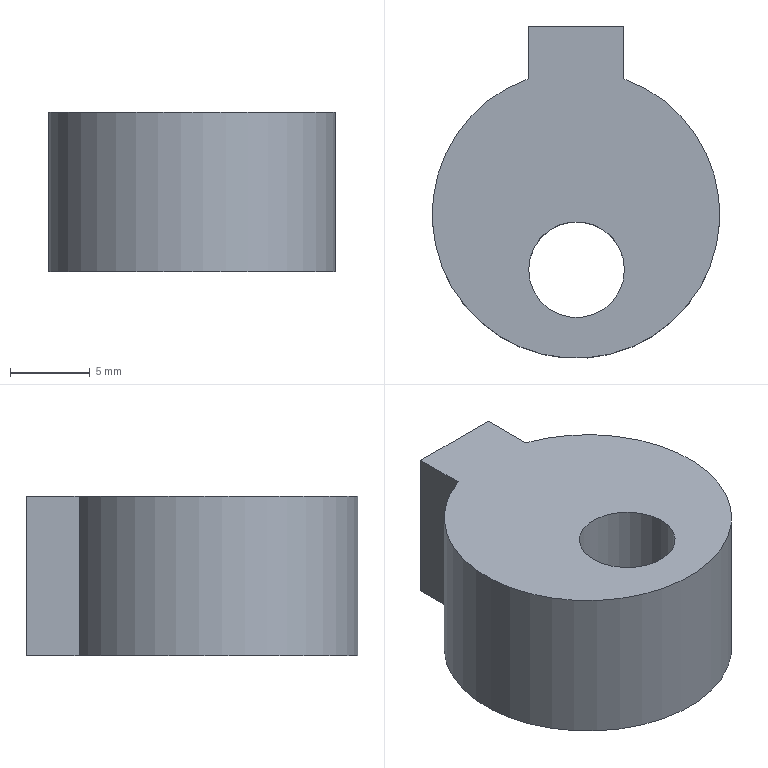NC program | NX | posted with a generic post | part box 18 x 20.8 x 10 mm
Lines 51 to 872 of 1937:
(动态粗 , TOOL : D6-18-D6-50-3T-FINISH)
N82 T05 M6
N84 G53
N86 G17 G0 G90 X-25.089 Y-2.254 S4500 M3
N88 G43 Z20. H5
N90 Z-11.5
N92 G94 G1 X-25.064 Y-2.255 Z-11.656 F2000.
N94 X-25.039 Y-2.257 Z-11.718
N96 X-25.014 Y-2.258 Z-11.763
N98 X-24.989 Y-2.26 Z-11.8
N100 X-24.964 Y-2.261 Z-11.831
N102 X-24.939 Y-2.263 Z-11.857
N104 X-24.914 Y-2.264 Z-11.88
N106 X-24.889 Y-2.265 Z-11.9
N108 X-24.864 Y-2.267 Z-11.918
N110 X-24.839 Y-2.268 Z-11.933
N112 X-24.814 Y-2.27 Z-11.947
N114 X-24.789 Y-2.271 Z-11.958
N116 X-24.764 Y-2.273 Z-11.968
N118 X-24.739 Y-2.274 Z-11.977
N120 X-24.714 Y-2.275 Z-11.984
N122 X-24.69 Y-2.277 Z-11.99
N124 X-24.665 Y-2.278 Z-11.994
N126 X-24.64 Y-2.28 Z-11.997
N128 X-24.615 Y-2.281 Z-11.999
N130 X-24.59 Y-2.283 Z-12.
N132 X-23.634 Y-2.337
N134 G3 X-23.007 Y-1.858 R0.606
N136 X-22.771 Y0.841 R12.318
N138 G1 X-22.75 Y5.629
N140 X-22.748 Y33.885
N142 G2 X-20.942 Y36.728 R3.519
N144 X-17.718 Y37.635 R7.361
N146 X-11.552 Y37.75 R85.996
N148 G1 X18.827 Y37.749
N150 G2 X21.708 Y35.989 R3.479
N152 X22.627 Y32.832 R7.163
N154 X22.749 Y27.585 R67.176
N156 G1 X22.75 Y-33.812
N158 G2 X21.024 Y-36.678 R3.471
N160 X17.814 Y-37.626 R7.137
N162 X12.585 Y-37.748 R66.821
N164 G1 X-18.813 Y-37.749
N166 G2 X-21.692 Y-36.003 R3.477
N168 X-22.624 Y-32.843 R7.13
N170 X-22.749 Y-27.578 R65.611
N172 G1 X-22.75 Y-3.315
N174 G3 X-22.536 Y0.764 R327.136
N176 G1 X-22.5 Y5.929
N178 X-22.498 Y32.723
N180 G2 X-19.99 Y36.522 R4.375
N182 X-16.46 Y37.385 R9.22
N184 X-10.181 Y37.499 R95.639
N186 G1 X17.645
N188 G2 X21.489 Y35.061 R4.343
N190 X22.38 Y31.54 R8.994
N192 X22.5 Y25.092 R94.03
N194 G1 Y-32.632
N196 G2 X20.044 Y-36.493 R4.354
N198 X16.427 Y-37.387 R9.188
N200 X10.635 Y-37.498 R90.52
N202 G1 X-17.634 Y-37.499
N204 G2 X-21.476 Y-35.077 R4.346
N206 X-22.38 Y-31.521 R8.993
N208 X-22.499 Y-25.186 R92.409
N210 G1 X-22.5 Y-4.366
N212 G2 X-22.302 Y0.513 R216.841
N214 G3 X-22.25 Y7.523 R427.399
N216 G1 X-22.248 Y31.71
N218 G2 X-19.268 Y36.282 R4.952
N220 X-15.484 Y37.136 R10.588
N222 X-9.543 Y37.249 R97.504
N224 G1 X16.576
N226 G2 X21.292 Y34.255 R4.957
N228 X22.132 Y30.545 R10.527
N230 X22.25 Y23.947 R104.773
N232 G1 Y-31.563
N234 G2 X19.203 Y-36.312 R4.973
N236 X15.355 Y-37.144 R10.934
N238 X7.913 Y-37.248 R134.719
N240 G1 X-16.677
N242 G2 X-21.298 Y-34.235 R4.957
N244 X-22.137 Y-30.466 R10.686
N246 X-22.249 Y-23.418 R117.87
N248 G1 Y-5.284
N250 G2 X-22.061 Y0.419 R175.91
N252 G3 X-22. Y7.935 R386.233
N254 G1 X-21.999 Y30.754
N256 G2 X-20.34 Y34.928 R5.437
N258 X-16.68 Y36.637 R7.255
N260 X-12.011 Y36.98 R27.631
N262 G1 X-6.649 Y36.999
N264 X15.789 Y36.997
N266 G2 X21.102 Y33.5 R5.439
N268 X21.898 Y29.49 R12.327
N270 X22. Y21.504 R157.622
N272 G1 X21.999 Y-30.795
N274 G2 X18.544 Y-36.08 R5.432
N276 X14.52 Y-36.894 R12.171
N278 X6.478 Y-36.998 R155.425
N280 G1 X-15.815 Y-36.997
N282 G2 X-21.094 Y-33.513 R5.437
N284 X-21.893 Y-29.562 R12.167
N286 X-21.999 Y-21.97 R140.366
N288 G1 Y-5.622
N290 G2 X-21.796 Y1.223 R364.638
N292 G3 X-21.75 Y8.366 R600.072
N294 G1 X-21.749 Y29.816
N296 G2 X-21.101 Y33.093 R6.845
N298 X-17.518 Y36.005 R6.131
N300 X-13.309 Y36.671 R15.33
N302 X-5.679 Y36.749 R207.213
N304 G1 X14.945 Y36.747
N306 G2 X18.403 Y35.93 R6.452
N308 X21.094 Y32.252 R6.331
N310 X21.686 Y27.992 R16.951
N312 X21.75 Y20.549 R265.611
N314 G1 X21.749 Y-29.951
N316 G2 X20.897 Y-33.455 R6.414
N318 X17.274 Y-36.084 R6.344
N320 X12.958 Y-36.685 R16.973
N322 X5.534 Y-36.748 R271.964
N324 G1 X-14.952 Y-36.747
N326 G2 X-18.474 Y-35.884 R6.407
N328 X-21.111 Y-32.187 R6.389
N330 X-21.695 Y-27.737 R17.838
N332 X-21.749 Y-21.344 R321.74
N334 G1 X-21.748 Y-6.091
N336 G2 X-21.545 Y1.444 R417.463
N338 G3 X-21.5 Y8.854 R609.069
N340 G1 X-21.499 Y29.085
N342 G2 X-20.955 Y32.371 R7.929
N344 X-17.271 Y35.653 R6.241
N346 X-13.039 Y36.399 R14.692
N348 X-4.865 Y36.499 R175.351
N350 G1 X14.12 Y36.497
N352 G2 X17.42 Y35.934 R7.805
N354 X20.647 Y32.289 R6.241
N356 X21.409 Y27.871 R14.999
N358 X21.499 Y19.697 R195.356
N360 G1 Y-29.107
N362 G2 X20.945 Y-32.392 R7.839
N364 X17.314 Y-35.635 R6.227
N366 X12.954 Y-36.403 R14.757
N368 X5.118 Y-36.498 R176.093
N370 G1 X-14.128 Y-36.497
N372 G2 X-17.427 Y-35.929 R7.774
N374 X-20.663 Y-32.241 R6.261
N376 X-21.409 Y-27.857 R15.14
N378 X-21.499 Y-19.89 R191.065
N380 G1 X-21.498 Y-6.541
N382 G2 X-21.291 Y1.85 R524.294
N384 G3 X-21.251 Y8.835 R604.453
N386 G1 X-21.25 Y28.279
N388 G2 X-20.846 Y31.519 R9.701
N390 X-17.052 Y35.297 R6.328
N392 X-12.649 Y36.134 R14.392
N394 X-4.063 Y36.249 R165.726
N396 G1 X13.389 Y36.247
N398 G2 X16.658 Y35.797 R9.171
N400 X20.327 Y31.978 R6.366
N402 X21.132 Y27.699 R14.476
N404 X21.249 Y20.426 R134.85
N406 G1 Y-28.17
N408 G2 X20.893 Y-31.38 R10.314
N410 X17.115 Y-35.27 R6.29
N412 X12.679 Y-36.131 R14.201
N414 X3.981 Y-36.248 R166.211
N416 G1 X-13.396 Y-36.247
N418 G2 X-16.717 Y-35.773 R9.053
N420 X-20.335 Y-31.953 R6.384
N422 X-21.136 Y-27.618 R14.689
N424 X-21.249 Y-18.957 R169.41
N426 G1 X-21.248 Y-7.178
N428 G2 X-21.045 Y1.757 R457.146
N430 G3 X-21.001 Y9.36 R617.01
N432 G1 X-21. Y27.417
N434 G2 X-20.707 Y30.675 R12.446
N436 X-16.812 Y34.955 R6.445
N438 X-12.367 Y35.864 R14.055
N440 X-4.945 Y35.998 R122.611
N442 G1 X12.32
N444 G2 X15.545 Y35.741 R13.358
N446 X19.937 Y31.857 R6.422
N448 X20.851 Y27.548 R13.659
N450 X20.998 Y19.844 R116.787
N452 G1 X20.999 Y-27.307
N454 G2 X20.735 Y-30.569 R13.277
N456 X16.826 Y-34.948 R6.434
N458 X12.419 Y-35.859 R13.955
N460 X4.847 Y-35.997 R122.098
N462 G1 X-12.328 Y-35.998
N464 G2 X-15.643 Y-35.715 R12.932
N466 X-19.953 Y-31.814 R6.44
N468 X-20.86 Y-27.426 R13.953
N470 X-20.998 Y-19.835 R121.849
N472 G1 Y-8.172
N474 G2 X-20.803 Y1.498 R375.98
N476 G3 X-20.751 Y9.66 R625.19
N478 G1 X-20.75 Y26.798
N480 G2 X-20.471 Y30.152 R13.814
N482 X-16.384 Y34.698 R6.633
N484 X-11.918 Y35.607 R14.471
N486 X-4.345 Y35.747 R121.858
N488 G1 X11.626 Y35.748
N490 G2 X14.986 Y35.51 R15.369
N492 X19.683 Y31.424 R6.615
N494 X20.598 Y27.037 R14.197
N496 X20.748 Y19.315 R117.436
N498 G1 X20.749 Y-26.614
N500 G2 X20.501 Y-30.028 R15.165
N502 X16.434 Y-34.676 R6.614
N504 X11.934 Y-35.604 R14.355
N506 X4.305 Y-35.747 R121.795
N508 G1 X-11.634
N510 G2 X-15.066 Y-35.491 R14.887
N512 X-19.688 Y-31.407 R6.621
N514 X-20.602 Y-26.981 R14.315
N516 X-20.747 Y-20.122 R106.439
N518 G1 X-20.748 Y-17.647
N520 G2 X-20.692 Y-3.716 R671.664
N522 G3 X-20.501 Y10.11 R372.941
N524 G1 X-20.5 Y26.048
N526 G2 X-20.262 Y29.52 R16.587
N528 X-16.087 Y34.395 R6.777
N530 X-11.593 Y35.342 R14.426
N532 X-4.096 Y35.497 R111.507
N534 G1 X10.952
N536 G2 X14.499 Y35.266 R17.187
N538 X19.418 Y31.034 R6.786
N540 X20.356 Y26.405 R14.872
N542 X20.498 Y18.982 R121.15
N544 G1 X20.499 Y-25.939
N546 G2 X20.273 Y-29.468 R17.424
N548 X16.042 Y-34.412 R6.785
N550 X11.469 Y-35.35 R14.752
N552 X3.578 Y-35.496 R125.286
N554 G1 X-10.94 Y-35.497
N556 G2 X-14.433 Y-35.279 R17.65
N558 X-19.394 Y-31.085 R6.774
N560 X-20.35 Y-26.479 R14.636
N562 X-20.497 Y-18.982 R117.855
N564 X-20.449 Y-4.169 R855.386
N566 G3 X-20.251 Y10.298 R406.187
N568 G1 X-20.25 Y25.56
N570 G2 X-20.001 Y29.126 R17.111
N572 X-15.761 Y34.109 R6.922
N574 X-11.121 Y35.089 R14.729
N576 X-3.361 Y35.247 R116.54
N578 G1 X10.483
N580 G2 X14.124 Y35.001 R17.48
N582 X19.146 Y30.675 R6.939
N584 X20.089 Y26.14 R14.873
N586 X20.247 Y18.456 R114.368
N588 G1 X20.248 Y-25.47
N590 G2 X20. Y-29.129 R17.469
N592 X15.716 Y-34.126 R6.931
N594 X11.016 Y-35.096 R15.007
N596 X3.65 Y-35.246 R115.969
N598 G1 X1.382 Y-35.247
N600 X-10.884 Y-35.246
N602 G2 X-14.459 Y-34.919 R14.171
N604 X-19.12 Y-30.732 R6.931
N606 X-20.087 Y-26.146 R14.752
N608 X-20.247 Y-18.462 R113.773
N610 X-20.177 Y-3.369 R660.883
N612 G3 X-20.002 Y9.904 R403.433
N614 G1 X-20. Y24.923
N616 G2 X-19.767 Y28.621 R19.176
N618 X-15.352 Y33.863 R7.08
N620 X-10.652 Y34.838 R15.219
N622 X-2.818 Y34.996 R118.686
N624 G1 X9.827 Y34.997
N626 G2 X13.601 Y34.769 R19.831
N628 X18.86 Y30.36 R7.073
N630 X19.84 Y25.641 R15.215
N632 X19.997 Y18.107 R115.058
N634 G1 X19.998 Y15.632
N636 Y-25.226
N638 G2 X19.704 Y-28.9 R16.149
N640 X15.305 Y-33.88 R7.088
N642 X10.546 Y-34.845 R15.51
N644 X3.124 Y-34.995 R118.018
N646 G1 X0.649 Y-34.997
N648 G2 X-11.802 Y-34.968 R745.044
N650 X-15.847 Y-33.933 R8.507
N652 X-19.097 Y-29.728 R7.525
N654 X-19.886 Y-24.912 R18.147
N656 X-19.998 Y-15.633 R203.304
N658 X-19.802 Y1.922 R507.437
N660 G3 X-19.752 Y9.923 R628.834
N662 G1 X-19.75 Y24.285
N664 G2 X-19.526 Y28.154 R21.29
N666 X-14.959 Y33.614 R7.225
N668 X-10.221 Y34.585 R15.61
N670 X-2.462 Y34.746 R117.444
N672 G1 X-0.193 Y34.747
N674 G2 X11.364 Y34.716 R634.778
N676 X15.404 Y33.725 R8.859
N678 X18.795 Y29.486 R7.58
N680 X19.623 Y24.679 R17.759
N682 X19.748 Y16.112 R168.234
N684 G1 Y-24.157
N686 G2 X19.544 Y-28.047 R22.865
N688 X15.002 Y-33.595 R7.214
N690 X10.209 Y-34.585 R15.56
N692 X2.581 Y-34.745 R116.201
N694 G1 X0.106 Y-34.747
N696 G2 X-11.352 Y-34.716 R636.751
N698 X-15.35 Y-33.753 R8.914
N700 X-18.787 Y-29.502 R7.558
N702 X-19.629 Y-24.564 R17.95
N704 X-19.747 Y-15.697 R183.794
N706 X-19.55 Y2.089 R540.24
N708 G3 X-19.502 Y10.092 R631.831
N710 G1 X-19.501 Y23.629
N712 G2 X-19.299 Y27.613 R24.421
N714 X-14.668 Y33.327 R7.343
N716 X-9.896 Y34.325 R15.642
N718 X-2.137 Y34.495 R112.951
N720 X10.764 Y34.471 R804.587
N722 X14.716 Y33.64 R9.695
N724 X18.448 Y29.364 R7.54
N726 X19.353 Y24.534 R16.957
N728 X19.498 Y15.743 R151.855
N730 G1 Y-23.539
N732 G2 X19.303 Y-27.579 R25.375
N734 X14.657 Y-33.33 R7.344
N736 X9.96 Y-34.319 R15.555
N738 X2.22 Y-34.495 R109.581
N740 X-10.752 Y-34.471 R819.057
N742 X-14.74 Y-33.627 R9.683
N744 X-18.441 Y-29.377 R7.54
N746 X-19.346 Y-24.622 R16.764
N748 X-19.496 Y-17.199 R121.937
N750 X-19.294 Y2.572 R625.364
N752 G1 X-19.252 Y10.579
N754 X-19.251 Y23.216
N756 G2 X-19.031 Y27.311 R24.18
N758 X-14.27 Y33.087 R7.471
N760 X-9.459 Y34.075 R16.089
N762 X-2.187 Y34.244 R107.514
N764 X10.394 Y34.218 R752.272
N766 X14.416 Y33.359 R9.85
N768 X18.193 Y29. R7.663
N770 X19.106 Y24.037 R17.466
N772 X19.247 Y14.927 R163.748
N774 G1 X19.248 Y-23.173
N776 G2 X19.037 Y-27.268 R24.822
N778 X14.264 Y-33.088 R7.471
N780 X9.452 Y-34.074 R16.112
N782 X1.618 Y-34.245 R115.826
N784 X-10.363 Y-34.218 R765.219
N786 X-14.388 Y-33.371 R9.923
N788 X-18.17 Y-29.058 R7.64
N790 X-19.097 Y-24.156 R17.108
N792 X-19.246 Y-16.602 R126.927
N794 X-19.045 Y2.628 R638.612
N796 G3 X-19.002 Y11.254 R658.402
N798 G1 X-19.001 Y22.504
N800 G2 X-18.814 Y26.715 R28.987
N802 X-13.953 Y32.818 R7.59
N804 X-9.143 Y33.816 R16.16
N806 X-1.722 Y33.994 R106.056
N808 X10.09 Y33.962 R566.408
N810 X14.194 Y33.042 R9.842
N812 X17.929 Y28.669 R7.785
N814 X18.847 Y23.727 R17.548
N816 X18.996 Y15.968 R132.2
N818 G1 X18.998 Y13.493
N820 X18.997 Y-23.032
N822 G2 X18.751 Y-27.069 R22.23
N824 X13.999 Y-32.796 R7.557
N826 X9.155 Y-33.814 R16.046
N828 X0.984 Y-33.994 R115.849
N830 X-10.078 Y-33.962 R508.437
N832 X-14.149 Y-33.064 R9.904
N834 X-17.936 Y-28.645 R7.788
N836 X-18.851 Y-23.664 R17.731
N838 X-18.997 Y-14.536 R161.107
N840 X-18.797 Y2.572 R628.619
N842 G3 X-18.752 Y11.198 R657.462
N844 G2 X-18.719 Y24.566 R796.512
N846 X-17.893 Y28.637 R10.532
N848 X-13.407 Y32.641 R7.823
N850 X-8.358 Y33.593 R17.611
N852 X-0.523 Y33.745 R132.044
N854 X9.695 Y33.71 R437.873
N856 X13.838 Y32.795 R10.103
N858 X17.674 Y28.32 R7.884
N860 X18.591 Y23.397 R17.729
N862 X18.746 Y15.525 R130.46
N864 G1 X18.747 Y13.05
N866 X18.746 Y-22.725
N868 G2 X18.482 Y-26.779 R21.671
N870 X13.66 Y-32.539 R7.66
N872 X8.759 Y-33.562 R16.327
N874 X0.513 Y-33.744 R117.382
N876 X-9.743 Y-33.707 R408.237
N878 X-13.898 Y-32.764 R9.97
N880 X-17.648 Y-28.384 R7.873
N882 X-18.583 Y-23.501 R17.393
N884 X-18.745 Y-15.742 R122.74
N886 X-18.546 Y2.683 R665.645
N888 G3 X-18.502 Y18.473 R944.618
N890 G2 X-18.43 Y24.865 R120.483
N892 X-17.147 Y29.206 R9.071
N894 X-12.757 Y32.496 R8.229
N896 X-7.727 Y33.357 R19.163
N898 X1.552 Y33.496 R175.224
N900 X9.539 Y33.447 R234.868
N902 X13.783 Y32.396 R9.752
N904 X17.406 Y28.013 R8.022
N906 X18.345 Y22.921 R18.117
N908 X18.497 Y13.812 R158.148
N910 G1 Y-21.57
N912 G2 X18.304 Y-25.986 R30.81
N914 X13.297 Y-32.293 R7.792
N916 X8.263 Y-33.319 R16.836
N918 X0.092 Y-33.494 R121.793
N920 X-9.433 Y-33.452 R332.693
N922 X-13.586 Y-32.498 R10.075
N924 X-17.388 Y-28.053 R7.967
N926 X-18.343 Y-22.946 R17.982
N928 X-18.496 Y-13.836 R156.067
N930 X-18.295 Y2.832 R699.402
N932 G3 X-18.253 Y17.704 R899.791
N934 G2 X-18.186 Y24.378 R136.775
N936 X-16.997 Y28.712 R9.494
N938 X-12.525 Y32.204 R8.229
N940 X-7.387 Y33.102 R19.079
N942 X1.367 Y33.245 R161.376
N944 X9.184 Y33.194 R209.128
N946 X13.43 Y32.154 R9.945
N948 X17.153 Y27.669 R8.105
N950 X18.087 Y22.635 R18.22
N952 X18.245 Y14.8 R129.788
N954 G1 X18.247 Y12.119
N956 X18.246 Y-21.706
N958 G2 X17.987 Y-26.005 R24.237
N960 X13.044 Y-32.004 R7.846
N962 X8.111 Y-33.049 R16.53
N964 X-0.172 Y-33.243 R113.221
N966 X-8.965 Y-33.204 R323.975
N968 X-13.166 Y-32.287 R10.507
N970 X-17.099 Y-27.808 R8.009
N972 X-18.082 Y-22.688 R17.805
N974 X-18.244 Y-14.816 R127.123
N976 X-18.045 Y2.962 R729.892
N978 G3 X-18.003 Y16.935 R866.975
N980 G2 X-17.934 Y24.003 R151.703
N982 X-16.778 Y28.329 R9.727
N984 X-12.26 Y31.925 R8.271
N986 X-7.164 Y32.841 R18.86
N988 X2.02 Y32.995 R159.327
N990 X8.994 Y32.931 R151.019
N992 X13.323 Y31.78 R9.734
N994 X16.929 Y27.25 R8.268
N996 X17.84 Y22.191 R18.824
N998 X17.996 Y12.912 R159.494
N1000 G1 X17.997 Y-20.594
N1002 G2 X17.804 Y-25.236 R33.839
N1004 X12.604 Y-31.793 R7.992
N1006 X7.512 Y-32.815 R17.404
N1008 X-0.866 Y-32.994 R125.319
N1010 X-8.853 Y-32.939 R206.629
N1012 X-13.166 Y-31.866 R10.037
N1014 X-16.907 Y-27.308 R8.215
N1016 X-17.837 Y-22.215 R18.653
N1018 X-17.996 Y-13.105 R154.344
N1020 X-17.789 Y3.539 R876.55
N1022 G3 X-17.753 Y16.166 R830.239
N1024 G2 X-17.687 Y23.571 R170.912
N1026 X-16.588 Y27.896 R10.078
N1028 X-12.048 Y31.628 R8.285
N1030 X-6.958 Y32.578 R18.519
N1032 X0.989 Y32.743 R128.438
N1034 X8.47 Y32.689 R182.514
N1036 X12.741 Y31.668 R10.345
N1038 X16.611 Y27.093 R8.229
N1040 X17.578 Y21.97 R18.38
N1042 X17.746 Y12.898 R146.75
N1044 G1 Y-20.121
N1046 G2 X17.567 Y-24.783 R36.372
N1048 X12.325 Y-31.519 R8.083
N1050 X7.217 Y-32.558 R17.414
N1052 X-0.954 Y-32.743 R118.986
N1054 X-8.435 Y-32.69 R189.266
N1056 X-12.693 Y-31.691 R10.438
N1058 X-16.605 Y-27.106 R8.215
N1060 X-17.574 Y-22.02 R18.253
N1062 X-17.745 Y-13.324 R136.639
N1064 X-17.539 Y3.558 R891.943
N1066 G3 X-17.503 Y15.398 R793.142
N1068 G2 X-17.441 Y23.122 R195.596
N1070 X-16.404 Y27.446 R10.494
N1072 X-11.855 Y31.324 R8.284
N1074 X-6.661 Y32.322 R18.315
N1076 X1.285 Y32.493 R125.355
N1078 X8.334 Y32.424 R138.718
N1080 X12.716 Y31.255 R9.983
N1082 X16.375 Y26.719 R8.383
N1084 X17.334 Y21.498 R18.942
N1086 X17.496 Y12.408 R153.697
N1088 G1 Y-19.617
N1090 G2 X17.313 Y-24.448 R37.822
N1092 X14.558 Y-29.756 R8.192
N1094 X9.835 Y-31.904 R10.493
N1096 X3.98 Y-32.442 R33.341
N1098 X-7.963 Y-32.445 R277.843
N1100 X-12.203 Y-31.522 R10.968
N1102 X-16.308 Y-26.894 R8.228
N1104 X-17.319 Y-21.703 R18.142
N1106 X-17.494 Y-13.119 R132.664
N1108 X-17.291 Y3.521 R914.552
N1110 G3 X-17.252 Y18.641 R963.899
N1112 G2 X-17.111 Y23.718 R51.731
N1114 X-15.28 Y28.463 R8.821
N1116 X-10.659 Y31.364 R9.152
N1118 X-5.232 Y32.134 R23.403
N1120 X7.535 Y32.197 R241.172
N1122 X11.822 Y31.3 R11.336
N1124 X16.021 Y26.661 R8.26
N1126 X17.06 Y21.458 R17.954
N1128 X17.244 Y13.211 R122.79
N1130 G1 X17.246 Y10.118
N1132 X17.245 Y-19.751
N1134 G2 X17.021 Y-24.372 R31.012
N1136 X11.7 Y-31.004 R8.211
N1138 X6.647 Y-32.043 R17.556
N1140 X-1.636 Y-32.242 R114.65
N1142 X-8.028 Y-32.168 R113.81
N1144 X-12.46 Y-30.968 R10.034
N1146 X-16.113 Y-26.413 R8.465
N1148 X-17.079 Y-21.175 R19.073
N1150 X-17.243 Y-12.104 R149.149
N1152 X-17.039 Y3.726 R994.956
N1154 G3 X-17.002 Y18.173 R940.914
N1156 G2 X-16.857 Y23.399 R52.53
N1158 X-14.988 Y28.207 R8.893
N1160 X-10.355 Y31.105 R9.234
N1162 X-5.022 Y31.876 R23.237
N1164 X7.369 Y31.936 R197.809
N1166 X11.742 Y30.934 R10.97
N1168 X15.796 Y26.269 R8.389
N1170 X16.813 Y21.041 R18.447
N1172 X16.994 Y12.382 R132.448
N1174 G1 X16.996 Y9.701
N1176 X16.995 Y-19.324
N1178 G2 X16.771 Y-24.02 R32.035
N1180 X11.41 Y-30.739 R8.283
N1182 X6.248 Y-31.795 R17.784
N1184 X-2.204 Y-31.992 R119.267
N1186 X-7.976 Y-31.894 R79.174
N1188 X-12.515 Y-30.492 R9.603
N1190 X-15.93 Y-25.896 R8.709
N1192 X-16.835 Y-20.72 R20.004
N1194 X-16.991 Y-11.01 R163.929
N1196 X-16.795 Y3.353 R951.417
N1198 G3 X-16.751 Y18.66 R979.702
N1200 G2 X-16.549 Y23.508 R36.98
N1202 X-13.923 Y28.763 R8.462
N1204 X-9.196 Y31.07 R10.364
N1206 X-3.292 Y31.679 R31.046
N1208 X6.981 Y31.687 R191.434
N1210 X11.314 Y30.738 R11.328
N1212 X15.502 Y26.059 R8.403
N1214 X16.545 Y20.911 R18.032
N1216 X16.742 Y13.077 R111.072
N1218 G1 X16.746 Y9.365
N1220 X16.745 Y-19.06
N1222 G2 X16.511 Y-23.737 R31.293
N1224 X11.119 Y-30.476 R8.344
N1226 X6.033 Y-31.533 R17.7
N1228 X-2.249 Y-31.741 R111.805
N1230 X-7.871 Y-31.62 R64.532
N1232 X-12.555 Y-30.002 R9.306
N1234 X-15.752 Y-25.352 R8.993
N1236 X-16.605 Y-20.015 R21.641
N1238 X-16.733 Y-9.386 R197.865
N1240 X-16.55 Y3.018 R921.774
N1242 G3 X-16.5 Y18.698 R987.207
N1244 G2 X-16.25 Y23.486 R31.079
N1246 X-10.876 Y30.197 R8.394
N1248 X-5.662 Y31.285 R17.792
N1250 X3.033 Y31.492 R118.621
N1252 X8.089 Y31.305 R40.379
N1254 X13.182 Y28.968 R8.663
N1256 X15.735 Y24.217 R9.978
N1258 X16.415 Y18.379 R28.301
N1260 X16.496 Y8.892 R344.157
N1262 G1 X16.494 Y-18.652
N1264 G2 X16.263 Y-23.385 R32.255
N1266 X10.843 Y-30.208 R8.406
N1268 X5.574 Y-31.291 R18.022
N1270 X-3.01 Y-31.491 R120.69
N1272 X-8.084 Y-31.305 R40.778
N1274 X-13.197 Y-28.95 R8.662
N1276 X-15.735 Y-24.21 R9.992
N1278 X-16.414 Y-18.372 R28.315
N1280 X-16.356 Y-0.566 R381.827
N1282 G3 X-16.249 Y18.736 R957.759
N1284 G2 X-15.968 Y23.334 R27.61
N1286 X-10.573 Y29.941 R8.446
N1288 X-5.343 Y31.032 R17.918
N1290 X3.446 Y31.24 R117.75
N1292 X8.234 Y30.981 R29.837
N1294 X14.92 Y25.625 R8.435
N1296 X16.028 Y20.398 R17.714
N1298 X16.241 Y12.302 R108.368
N1300 G1 X16.245 Y8.59
N1302 X16.244 Y-18.223
N1304 G2 X16.021 Y-22.994 R33.946
N1306 X13.099 Y-28.455 R8.503
N1308 X8.377 Y-30.602 R10.87
N1310 X2.432 Y-31.181 R33.116
N1312 X-6.547 Y-31.169 R135.689
N1314 X-10.962 Y-30.101 R10.996
N1316 X-15.013 Y-25.385 R8.584
N1318 X-16.041 Y-20.235 R18.522
N1320 X-16.238 Y-11.577 R118.864
N1322 X-16.045 Y3.539 R975.523
N1324 G3 X-15.999 Y18.229 R966.899
N1326 G2 X-15.72 Y22.997 R28.979
N1328 X-10.294 Y29.677 R8.504
N1330 X-4.991 Y30.782 R18.078
N1332 X6.253 Y30.915 R112.994
N1334 X10.67 Y29.844 R11.077
N1336 X14.739 Y25.138 R8.622
N1338 X15.784 Y19.971 R18.435
N1340 X15.99 Y12.138 R108.831
N1342 G1 X15.995 Y8.013
N1344 X15.994 Y-17.824
N1346 G2 X15.763 Y-22.708 R34.27
N1348 X12.808 Y-28.199 R8.557
N1350 X8.007 Y-30.361 R11.004
N1352 X1.892 Y-30.936 R34.455
N1354 X-6.281 Y-30.913 R116.945
N1356 X-10.742 Y-29.805 R10.962
N1358 X-14.758 Y-25.084 R8.653
N1360 X-15.797 Y-19.803 R18.863
N1362 X-15.984 Y-10.488 R129.95
N1364 X-15.796 Y3.539 R996.132
N1366 G3 X-15.749 Y17.967 R957.371
N1368 G2 X-15.474 Y22.641 R29.161
N1370 X-10.012 Y29.415 R8.563
N1372 X-4.709 Y30.527 R18.1
N1374 X6.121 Y30.65 R97.929
N1376 X10.667 Y29.432 R10.674
N1378 X14.517 Y24.752 R8.759
N1380 X15.545 Y19.488 R19.056
N1382 X15.743 Y10.699 R128.415
N1384 G1 X15.745 Y7.605
N1386 X15.744 Y-17.37
N1388 G2 X15.52 Y-22.33 R36.138
N1390 X12.85 Y-27.656 R8.709
N1392 X8.113 Y-30.014 R10.525
N1394 X2.233 Y-30.664 R30.17
N1396 X-5.94 Y-30.662 R107.488
N1398 X-10.456 Y-29.545 R11.089
N1400 X-14.496 Y-24.803 R8.704
N1402 X-15.538 Y-19.561 R18.813
N1404 X-15.734 Y-10.902 R117.491
N1406 X-15.546 Y3.558 R988.97
N1408 G3 X-15.498 Y17.742 R933.373
N1410 G2 X-15.197 Y22.47 R27.723
N1412 X-9.759 Y29.142 R8.599
N1414 X-4.553 Y30.261 R17.862
N1416 X5.771 Y30.399 R89.365
N1418 X10.292 Y29.223 R10.885
N1420 X14.247 Y24.493 R8.782
N1422 X15.292 Y19.176 R19.096
N1424 X15.493 Y10.311 R129.009
N1426 G1 X15.495 Y7.217
N1428 X15.494 Y-16.989
N1430 G2 X15.275 Y-21.968 R37.318
N1432 X12.756 Y-27.22 R8.842
N1434 X7.93 Y-29.73 R10.376
N1436 X2.073 Y-30.407 R29.27
N1438 X-5.874 Y-30.391 R87.703
N1440 X-10.415 Y-29.153 R10.657
N1442 X-14.281 Y-24.4 R8.844
N1444 X-15.299 Y-19.074 R19.512
N1446 X-15.478 Y-9.797 R129.798
N1448 X-15.304 Y2.942 R917.359
N1450 G3 X-15.245 Y17.761 R997.288
N1452 G2 X-14.904 Y22.373 R24.827
N1454 X-9.51 Y28.869 R8.626
N1456 X-4.213 Y30.011 R17.938
N1458 X5.604 Y30.135 R78.322
N1460 X10.21 Y28.85 R10.62
N1462 X14.036 Y24.082 R8.917
N1464 X15.052 Y18.701 R19.798
N1466 X15.242 Y10.043 R133.104
N1468 G1 X15.245 Y6.949
N1470 X15.244 Y-16.582
N1472 G2 X15.026 Y-21.636 R38.384
N1474 X12.596 Y-26.844 R8.948
N1476 X7.774 Y-29.44 R10.265
N1478 X1.978 Y-30.147 R28.137
N1480 X-5.706 Y-30.126 R75.476
N1482 X-10.311 Y-28.789 R10.435
N1484 X-14.053 Y-24.03 R8.964
N1486 X-15.054 Y-18.664 R20.011
N1488 X-15.222 Y-8.973 R136.693
N1490 G1 X-15.041 Y4.192
N1492 X-14.987 Y18.08
N1494 G2 X-14.548 Y22.53 R20.149
N1496 X-9.228 Y28.609 R8.65
N1498 X-4.044 Y29.746 R17.797
N1500 X5.416 Y29.872 R68.952
N1502 X10.089 Y28.496 R10.439
N1504 X13.804 Y23.725 R9.032
N1506 X14.811 Y18.246 R20.371
N1508 X14.992 Y9.681 R138.402
N1510 G1 X14.994 Y6.587
N1512 X14.993 Y-16.213
N1514 G2 X14.769 Y-21.36 R38.576
N1516 X12.348 Y-26.555 R8.999
N1518 X7.511 Y-29.176 R10.288
N1520 X1.602 Y-29.898 R28.326
N1522 X-5.426 Y-29.87 R66.754
N1524 X-10.062 Y-28.51 R10.446
N1526 X-13.815 Y-23.69 R9.037
N1528 X-14.802 Y-18.358 R20.237
N1530 X-14.971 Y-9.08 R130.038
N1532 G1 X-14.791 Y4.211
N1534 X-14.734 Y17.874
N1536 G2 X-14.249 Y22.412 R19.234
N1538 X-9.023 Y28.319 R8.674
N1540 X-3.716 Y29.495 R17.772
N1542 X5.163 Y29.613 R62.075
N1544 X9.8 Y28.241 R10.458
N1546 X13.535 Y23.474 R9.056
N1548 X14.545 Y18.129 R20.016
N1550 X14.741 Y9.452 R130.401
N1552 G1 X14.744 Y6.564
N1554 X14.743 Y-15.823
N1556 G2 X14.531 Y-20.953 R40.5
N1558 X12.324 Y-26.029 R9.204
N1560 X7.459 Y-28.857 R10.037
N1562 X1.635 Y-29.632 R26.525
N1564 X-5.355 Y-29.594 R56.828
N1566 X-10.101 Y-28.048 R10.068
N1568 X-13.617 Y-23.238 R9.242
N1570 X-14.57 Y-17.766 R21.342
N1572 X-14.706 Y-7.363 R152.588
N1574 G1 X-14.542 Y4.248
N1576 X-14.494 Y16.862
N1578 G2 X-14.13 Y21.547 R24.686
N1580 X-8.665 Y28.093 R8.76
N1582 X-3.335 Y29.25 R18.152
N1584 X5.075 Y29.338 R53.937
N1586 X9.837 Y27.781 R10.097
N1588 X13.354 Y22.975 R9.278
N1590 X14.317 Y17.487 R21.337
N1592 X14.492 Y8.809 R146.672
N1594 G1 X14.494 Y5.715
N1596 X14.493 Y-15.435
N1598 G2 X14.285 Y-20.602 R41.912
N1600 X12.173 Y-25.631 R9.342
N1602 X7.402 Y-28.535 R9.889
N1604 X1.718 Y-29.361 R24.799
N1606 X-5.083 Y-29.337 R51.728
N1608 X-9.884 Y-27.747 R10.05
N1610 X-13.378 Y-22.9 R9.329
N1612 X-14.32 Y-17.427 R21.638
N1614 X-14.456 Y-7.511 R146.547
N1616 G1 X-14.292 Y4.304
N1618 X-14.233 Y17.237
N1620 G2 X-13.755 Y21.777 R19.785
N1622 X-8.413 Y27.824 R8.773
N1624 X-3.216 Y28.981 R17.862
N1626 X4.8 Y29.08 R48.917
N1628 X9.623 Y27.479 R10.084
N1630 X13.106 Y22.667 R9.345
N1632 X14.072 Y17.085 R21.699
N1634 X14.242 Y8.201 R154.698
N1636 G1 X14.244 Y5.313
N1638 X14.243 Y-15.031
N1640 G2 X14.032 Y-20.31 R42.683
N1642 X11.91 Y-25.36 R9.393
N1644 X7.024 Y-28.306 R9.985
N1646 X1.187 Y-29.12 R25.759
N1648 X-5.107 Y-29.047 R42.316
N1650 X-10.084 Y-27.137 R9.594
N1652 X-13.196 Y-22.391 R9.651
N1654 X-14.089 Y-16.776 R23.128
N1656 X-14.189 Y-6.054 R169.885
N1658 G3 X-13.994 Y16.169 R977.301
N1660 G2 X-13.619 Y20.984 R25.175
N1662 X-8.091 Y27.585 R8.847
N1664 X-2.758 Y28.743 R18.296
N1666 X4.713 Y28.802 R42.732
N1668 X9.63 Y27.017 R9.793
N1670 X12.928 Y22.149 R9.593
N1672 X13.84 Y16.462 R23.168
N1674 X13.993 Y7.183 R180.884
N1676 G1 X13.994 Y-13.817
N1678 G2 X13.839 Y-19.512 R61.049
N1680 X12.25 Y-24.306 R10.241
N1682 X7.481 Y-27.814 R9.343
N1684 X2.053 Y-28.799 R20.976
N1686 X-4.82 Y-28.789 R40.919
N1688 X-9.788 Y-26.894 R9.632
N1690 X-12.967 Y-22.02 R9.722
N1692 X-13.843 Y-16.383 R23.688
N1694 X-13.931 Y-5.566 R173.843
N1696 G3 X-13.743 Y15.907 R974.239
N1698 G2 X-13.368 Y20.685 R25.175
N1700 X-7.824 Y27.323 R8.886
N1702 X-2.55 Y28.483 R18.192
N1704 X4.602 Y28.524 R37.689
N1706 X9.719 Y26.471 R9.533
N1708 X12.754 Y21.606 R9.914
N1710 X13.604 Y15.888 R24.72
N1712 X13.743 Y5.165 R232.046
N1714 G1 Y-14.26
N1716 G2 X13.531 Y-19.689 R44.594
N1718 X11.447 Y-24.75 R9.55